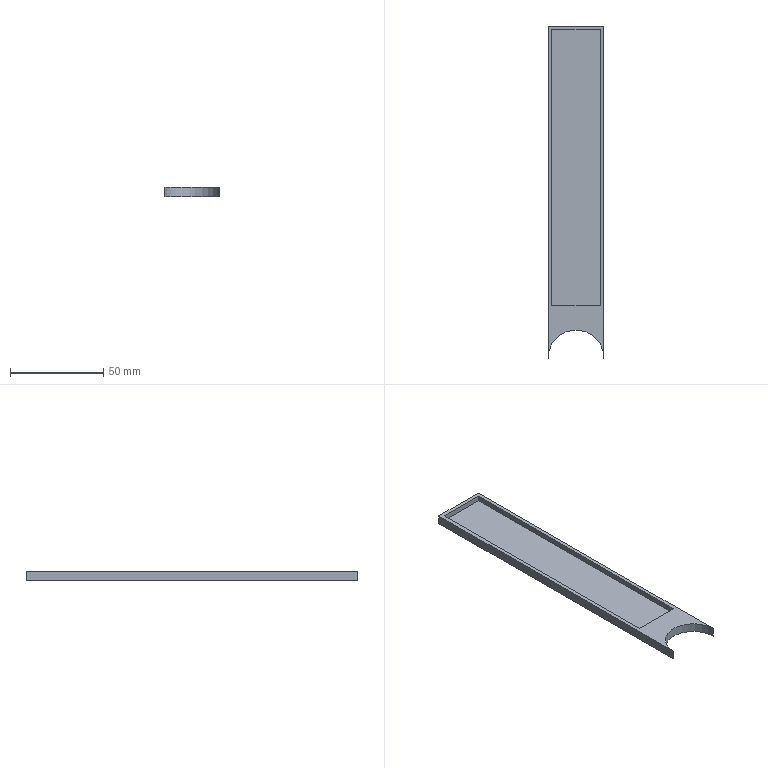Part | SolidWorks | features ICE 4, Extrusion 1 | 1 solid | 11 faces | box 30 x 178 x 5 mm | volume 13389 mm3 | plane 10 | cylinder 1 | commonest cylinder face diameters 30 x1
STEP:
#1=CARTESIAN_POINT('',(2.,28.,2.));
#2=VERTEX_POINT('',#1);
#3=CARTESIAN_POINT('',(28.,28.,2.));
#4=VERTEX_POINT('',#3);
#5=CARTESIAN_POINT('',(2.,28.,2.));
#6=DIRECTION('',(1.,0.,0.));
#7=VECTOR('',#6,1000.);
#8=LINE('',#5,#7);
#9=EDGE_CURVE('',#2,#4,#8,.T.);
#10=ORIENTED_EDGE('',*,*,#9,.T.);
#11=CARTESIAN_POINT('',(28.,176.,2.));
#12=VERTEX_POINT('',#11);
#13=CARTESIAN_POINT('',(28.,176.,2.));
#14=DIRECTION('',(0.,1.,0.));
#15=VECTOR('',#14,1000.);
#16=LINE('',#13,#15);
#17=EDGE_CURVE('',#4,#12,#16,.T.);
#18=ORIENTED_EDGE('',*,*,#17,.T.);
#19=CARTESIAN_POINT('',(2.,176.,2.));
#20=VERTEX_POINT('',#19);
#21=CARTESIAN_POINT('',(2.,176.,2.));
#22=DIRECTION('',(-1.,0.,0.));
#23=VECTOR('',#22,1000.);
#24=LINE('',#21,#23);
#25=EDGE_CURVE('',#12,#20,#24,.T.);
#26=ORIENTED_EDGE('',*,*,#25,.T.);
#27=CARTESIAN_POINT('',(2.,176.,2.));
#28=DIRECTION('',(0.,-1.,0.));
#29=VECTOR('',#28,1000.);
#30=LINE('',#27,#29);
#31=EDGE_CURVE('',#20,#2,#30,.T.);
#32=ORIENTED_EDGE('',*,*,#31,.T.);
#33=EDGE_LOOP('',(#10,#18,#26,#32));
#34=FACE_OUTER_BOUND('',#33,.T.);
#35=CARTESIAN_POINT('',(0.,0.,2.));
#36=DIRECTION('',(0.,0.,1.));
#37=DIRECTION('',(1.,0.,0.));
#38=AXIS2_PLACEMENT_3D('',#35,#36,#37);
#39=PLANE('',#38);
#40=ADVANCED_FACE('',(#34),#39,.T.);
#41=CARTESIAN_POINT('',(2.,176.,5.));
#42=VERTEX_POINT('',#41);
#43=CARTESIAN_POINT('',(2.,28.,5.));
#44=VERTEX_POINT('',#43);
#45=CARTESIAN_POINT('',(2.,176.,5.));
#46=DIRECTION('',(0.,-1.,0.));
#47=VECTOR('',#46,1000.);
#48=LINE('',#45,#47);
#49=EDGE_CURVE('',#42,#44,#48,.T.);
#50=ORIENTED_EDGE('',*,*,#49,.T.);
#51=CARTESIAN_POINT('',(2.,28.,32.857));
#52=DIRECTION('',(0.,0.,-1.));
#53=VECTOR('',#52,1000.);
#54=LINE('',#51,#53);
#55=EDGE_CURVE('',#44,#2,#54,.T.);
#56=ORIENTED_EDGE('',*,*,#55,.T.);
#57=ORIENTED_EDGE('',*,*,#31,.F.);
#58=CARTESIAN_POINT('',(2.,176.,2.));
#59=DIRECTION('',(0.,0.,1.));
#60=VECTOR('',#59,1000.);
#61=LINE('',#58,#60);
#62=EDGE_CURVE('',#20,#42,#61,.T.);
#63=ORIENTED_EDGE('',*,*,#62,.T.);
#64=EDGE_LOOP('',(#50,#56,#57,#63));
#65=FACE_OUTER_BOUND('',#64,.T.);
#66=CARTESIAN_POINT('',(2.,176.,2.));
#67=DIRECTION('',(-1.,0.,0.));
#68=DIRECTION('',(0.,-1.,0.));
#69=AXIS2_PLACEMENT_3D('',#66,#67,#68);
#70=PLANE('',#69);
#71=ADVANCED_FACE('',(#65),#70,.F.);
#72=ORIENTED_EDGE('',*,*,#17,.F.);
#73=CARTESIAN_POINT('',(28.,28.,5.));
#74=VERTEX_POINT('',#73);
#75=CARTESIAN_POINT('',(28.,28.,32.857));
#76=DIRECTION('',(0.,0.,-1.));
#77=VECTOR('',#76,1000.);
#78=LINE('',#75,#77);
#79=EDGE_CURVE('',#74,#4,#78,.T.);
#80=ORIENTED_EDGE('',*,*,#79,.F.);
#81=CARTESIAN_POINT('',(28.,176.,5.));
#82=VERTEX_POINT('',#81);
#83=CARTESIAN_POINT('',(28.,0.,5.));
#84=DIRECTION('',(0.,-1.,0.));
#85=VECTOR('',#84,1000.);
#86=LINE('',#83,#85);
#87=EDGE_CURVE('',#82,#74,#86,.T.);
#88=ORIENTED_EDGE('',*,*,#87,.F.);
#89=CARTESIAN_POINT('',(28.,176.,2.));
#90=DIRECTION('',(0.,0.,1.));
#91=VECTOR('',#90,1000.);
#92=LINE('',#89,#91);
#93=EDGE_CURVE('',#12,#82,#92,.T.);
#94=ORIENTED_EDGE('',*,*,#93,.F.);
#95=EDGE_LOOP('',(#72,#80,#88,#94));
#96=FACE_OUTER_BOUND('',#95,.T.);
#97=CARTESIAN_POINT('',(28.,176.,2.));
#98=DIRECTION('',(1.,0.,0.));
#99=DIRECTION('',(0.,1.,0.));
#100=AXIS2_PLACEMENT_3D('',#97,#98,#99);
#101=PLANE('',#100);
#102=ADVANCED_FACE('',(#96),#101,.F.);
#103=CARTESIAN_POINT('',(30.,0.,0.));
#104=VERTEX_POINT('',#103);
#105=CARTESIAN_POINT('',(30.,178.,0.));
#106=VERTEX_POINT('',#105);
#107=CARTESIAN_POINT('',(30.,178.,0.));
#108=DIRECTION('',(0.,1.,0.));
#109=VECTOR('',#108,1000.);
#110=LINE('',#107,#109);
#111=EDGE_CURVE('',#104,#106,#110,.T.);
#112=ORIENTED_EDGE('',*,*,#111,.T.);
#113=CARTESIAN_POINT('',(30.,178.,5.));
#114=VERTEX_POINT('',#113);
#115=CARTESIAN_POINT('',(30.,178.,5.));
#116=DIRECTION('',(0.,0.,-1.));
#117=VECTOR('',#116,1000.);
#118=LINE('',#115,#117);
#119=EDGE_CURVE('',#114,#106,#118,.T.);
#120=ORIENTED_EDGE('',*,*,#119,.F.);
#121=CARTESIAN_POINT('',(30.,0.,5.));
#122=VERTEX_POINT('',#121);
#123=CARTESIAN_POINT('',(30.,178.,5.));
#124=DIRECTION('',(0.,1.,0.));
#125=VECTOR('',#124,1000.);
#126=LINE('',#123,#125);
#127=EDGE_CURVE('',#122,#114,#126,.T.);
#128=ORIENTED_EDGE('',*,*,#127,.F.);
#129=CARTESIAN_POINT('',(30.,0.,5.));
#130=DIRECTION('',(0.,0.,-1.));
#131=VECTOR('',#130,1000.);
#132=LINE('',#129,#131);
#133=EDGE_CURVE('',#122,#104,#132,.T.);
#134=ORIENTED_EDGE('',*,*,#133,.T.);
#135=EDGE_LOOP('',(#112,#120,#128,#134));
#136=FACE_OUTER_BOUND('',#135,.T.);
#137=CARTESIAN_POINT('',(30.,178.,5.));
#138=DIRECTION('',(-1.,0.,0.));
#139=DIRECTION('',(0.,-1.,0.));
#140=AXIS2_PLACEMENT_3D('',#137,#138,#139);
#141=PLANE('',#140);
#142=ADVANCED_FACE('',(#136),#141,.F.);
#143=CARTESIAN_POINT('',(0.,178.,0.));
#144=VERTEX_POINT('',#143);
#145=CARTESIAN_POINT('',(30.,178.,0.));
#146=DIRECTION('',(-1.,0.,0.));
#147=VECTOR('',#146,1000.);
#148=LINE('',#145,#147);
#149=EDGE_CURVE('',#106,#144,#148,.T.);
#150=ORIENTED_EDGE('',*,*,#149,.T.);
#151=CARTESIAN_POINT('',(0.,178.,5.));
#152=VERTEX_POINT('',#151);
#153=CARTESIAN_POINT('',(0.,178.,5.));
#154=DIRECTION('',(0.,0.,-1.));
#155=VECTOR('',#154,1000.);
#156=LINE('',#153,#155);
#157=EDGE_CURVE('',#152,#144,#156,.T.);
#158=ORIENTED_EDGE('',*,*,#157,.F.);
#159=CARTESIAN_POINT('',(30.,178.,5.));
#160=DIRECTION('',(-1.,0.,0.));
#161=VECTOR('',#160,1000.);
#162=LINE('',#159,#161);
#163=EDGE_CURVE('',#114,#152,#162,.T.);
#164=ORIENTED_EDGE('',*,*,#163,.F.);
#165=ORIENTED_EDGE('',*,*,#119,.T.);
#166=EDGE_LOOP('',(#150,#158,#164,#165));
#167=FACE_OUTER_BOUND('',#166,.T.);
#168=CARTESIAN_POINT('',(30.,178.,5.));
#169=DIRECTION('',(0.,-1.,0.));
#170=DIRECTION('',(1.,0.,0.));
#171=AXIS2_PLACEMENT_3D('',#168,#169,#170);
#172=PLANE('',#171);
#173=ADVANCED_FACE('',(#167),#172,.F.);
#174=CARTESIAN_POINT('',(0.,0.,0.));
#175=VERTEX_POINT('',#174);
#176=CARTESIAN_POINT('',(0.,178.,0.));
#177=DIRECTION('',(0.,-1.,0.));
#178=VECTOR('',#177,1000.);
#179=LINE('',#176,#178);
#180=EDGE_CURVE('',#144,#175,#179,.T.);
#181=ORIENTED_EDGE('',*,*,#180,.T.);
#182=CARTESIAN_POINT('',(0.,0.,5.));
#183=VERTEX_POINT('',#182);
#184=CARTESIAN_POINT('',(0.,0.,5.));
#185=DIRECTION('',(0.,0.,-1.));
#186=VECTOR('',#185,1000.);
#187=LINE('',#184,#186);
#188=EDGE_CURVE('',#183,#175,#187,.T.);
#189=ORIENTED_EDGE('',*,*,#188,.F.);
#190=CARTESIAN_POINT('',(0.,178.,5.));
#191=DIRECTION('',(0.,-1.,0.));
#192=VECTOR('',#191,1000.);
#193=LINE('',#190,#192);
#194=EDGE_CURVE('',#152,#183,#193,.T.);
#195=ORIENTED_EDGE('',*,*,#194,.F.);
#196=ORIENTED_EDGE('',*,*,#157,.T.);
#197=EDGE_LOOP('',(#181,#189,#195,#196));
#198=FACE_OUTER_BOUND('',#197,.T.);
#199=CARTESIAN_POINT('',(0.,178.,5.));
#200=DIRECTION('',(1.,0.,0.));
#201=DIRECTION('',(0.,1.,0.));
#202=AXIS2_PLACEMENT_3D('',#199,#200,#201);
#203=PLANE('',#202);
#204=ADVANCED_FACE('',(#198),#203,.F.);
#205=CARTESIAN_POINT('',(15.,0.,5.));
#206=DIRECTION('',(0.,0.,-1.));
#207=DIRECTION('',(-1.,0.,0.));
#208=AXIS2_PLACEMENT_3D('',#205,#206,#207);
#209=CIRCLE('',#208,15.);
#210=EDGE_CURVE('',#183,#122,#209,.T.);
#211=ORIENTED_EDGE('',*,*,#210,.T.);
#212=ORIENTED_EDGE('',*,*,#127,.T.);
#213=ORIENTED_EDGE('',*,*,#163,.T.);
#214=ORIENTED_EDGE('',*,*,#194,.T.);
#215=EDGE_LOOP('',(#211,#212,#213,#214));
#216=FACE_OUTER_BOUND('',#215,.T.);
#217=CARTESIAN_POINT('',(2.,28.,5.));
#218=DIRECTION('',(-1.,0.,0.));
#219=VECTOR('',#218,1000.);
#220=LINE('',#217,#219);
#221=EDGE_CURVE('',#74,#44,#220,.T.);
#222=ORIENTED_EDGE('',*,*,#221,.T.);
#223=ORIENTED_EDGE('',*,*,#49,.F.);
#224=CARTESIAN_POINT('',(2.,176.,5.));
#225=DIRECTION('',(-1.,0.,0.));
#226=VECTOR('',#225,1000.);
#227=LINE('',#224,#226);
#228=EDGE_CURVE('',#82,#42,#227,.T.);
#229=ORIENTED_EDGE('',*,*,#228,.F.);
#230=ORIENTED_EDGE('',*,*,#87,.T.);
#231=EDGE_LOOP('',(#222,#223,#229,#230));
#232=FACE_BOUND('',#231,.T.);
#233=CARTESIAN_POINT('',(0.,0.,5.));
#234=DIRECTION('',(0.,0.,-1.));
#235=DIRECTION('',(-1.,0.,0.));
#236=AXIS2_PLACEMENT_3D('',#233,#234,#235);
#237=PLANE('',#236);
#238=ADVANCED_FACE('',(#216,#232),#237,.F.);
#239=CARTESIAN_POINT('',(15.,0.,0.));
#240=DIRECTION('',(0.,0.,-1.));
#241=DIRECTION('',(-1.,0.,0.));
#242=AXIS2_PLACEMENT_3D('',#239,#240,#241);
#243=CIRCLE('',#242,15.);
#244=EDGE_CURVE('',#175,#104,#243,.T.);
#245=ORIENTED_EDGE('',*,*,#244,.F.);
#246=ORIENTED_EDGE('',*,*,#180,.F.);
#247=ORIENTED_EDGE('',*,*,#149,.F.);
#248=ORIENTED_EDGE('',*,*,#111,.F.);
#249=EDGE_LOOP('',(#245,#246,#247,#248));
#250=FACE_OUTER_BOUND('',#249,.T.);
#251=CARTESIAN_POINT('',(0.,0.,0.));
#252=DIRECTION('',(0.,0.,-1.));
#253=DIRECTION('',(-1.,0.,0.));
#254=AXIS2_PLACEMENT_3D('',#251,#252,#253);
#255=PLANE('',#254);
#256=ADVANCED_FACE('',(#250),#255,.T.);
#257=ORIENTED_EDGE('',*,*,#228,.T.);
#258=ORIENTED_EDGE('',*,*,#62,.F.);
#259=ORIENTED_EDGE('',*,*,#25,.F.);
#260=ORIENTED_EDGE('',*,*,#93,.T.);
#261=EDGE_LOOP('',(#257,#258,#259,#260));
#262=FACE_OUTER_BOUND('',#261,.T.);
#263=CARTESIAN_POINT('',(2.,176.,2.));
#264=DIRECTION('',(0.,1.,0.));
#265=DIRECTION('',(0.,0.,1.));
#266=AXIS2_PLACEMENT_3D('',#263,#264,#265);
#267=PLANE('',#266);
#268=ADVANCED_FACE('',(#262),#267,.F.);
#269=ORIENTED_EDGE('',*,*,#221,.F.);
#270=ORIENTED_EDGE('',*,*,#79,.T.);
#271=ORIENTED_EDGE('',*,*,#9,.F.);
#272=ORIENTED_EDGE('',*,*,#55,.F.);
#273=EDGE_LOOP('',(#269,#270,#271,#272));
#274=FACE_OUTER_BOUND('',#273,.T.);
#275=CARTESIAN_POINT('',(2.,28.,32.857));
#276=DIRECTION('',(0.,1.,0.));
#277=DIRECTION('',(0.,0.,1.));
#278=AXIS2_PLACEMENT_3D('',#275,#276,#277);
#279=PLANE('',#278);
#280=ADVANCED_FACE('',(#274),#279,.T.);
#281=ORIENTED_EDGE('',*,*,#244,.T.);
#282=ORIENTED_EDGE('',*,*,#133,.F.);
#283=ORIENTED_EDGE('',*,*,#210,.F.);
#284=ORIENTED_EDGE('',*,*,#188,.T.);
#285=EDGE_LOOP('',(#281,#282,#283,#284));
#286=FACE_OUTER_BOUND('',#285,.T.);
#287=CARTESIAN_POINT('',(15.,0.,7.));
#288=DIRECTION('',(0.,0.,-1.));
#289=DIRECTION('',(-1.,0.,0.));
#290=AXIS2_PLACEMENT_3D('',#287,#288,#289);
#291=CYLINDRICAL_SURFACE('',#290,15.);
#292=ADVANCED_FACE('',(#286),#291,.F.);
#293=CLOSED_SHELL('',(#40,#71,#102,#142,#173,#204,#238,#256,#268,#280,#292));
#294=MANIFOLD_SOLID_BREP('',#293);
#295=CARTESIAN_POINT('',(0.,0.,0.));
#296=DIRECTION('',(0.,0.,1.));
#297=DIRECTION('',(1.,0.,0.));
#298=AXIS2_PLACEMENT_3D('',#295,#296,#297);
#299=(LENGTH_UNIT()NAMED_UNIT(*)SI_UNIT(.MILLI.,.METRE.));
#300=UNCERTAINTY_MEASURE_WITH_UNIT(LENGTH_MEASURE(0.00001),#299,'','');
#301=(NAMED_UNIT(*)PLANE_ANGLE_UNIT()SI_UNIT($,.RADIAN.));
#302=(NAMED_UNIT(*)SI_UNIT($,.STERADIAN.)SOLID_ANGLE_UNIT());
#303=(GEOMETRIC_REPRESENTATION_CONTEXT(3)GLOBAL_UNCERTAINTY_ASSIGNED_CONTEXT((#300))GLOBAL_UNIT_ASSIGNED_CONTEXT((#299,#301,#302))REPRESENTATION_CONTEXT('',''));
#304=ADVANCED_BREP_SHAPE_REPRESENTATION('',(#294,#298),#303);